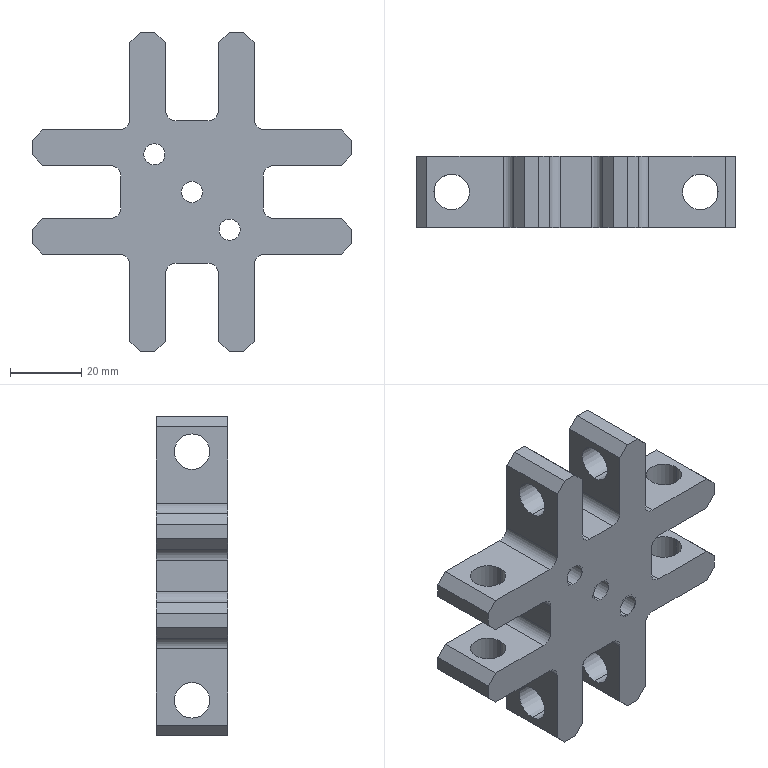Part | SolidWorks | features Chamfer 4, CirPattern 3, ICE 3, Fillet 2, HoleWzd 2, Extrusion 1 | 1 solid | 86 faces | box 90 x 20 x 90 mm | volume 62065 mm3 | plane 46 | cylinder 34 | cone 6 | commonest cylinder face diameters 10 x16 6 x12 6.8 x6